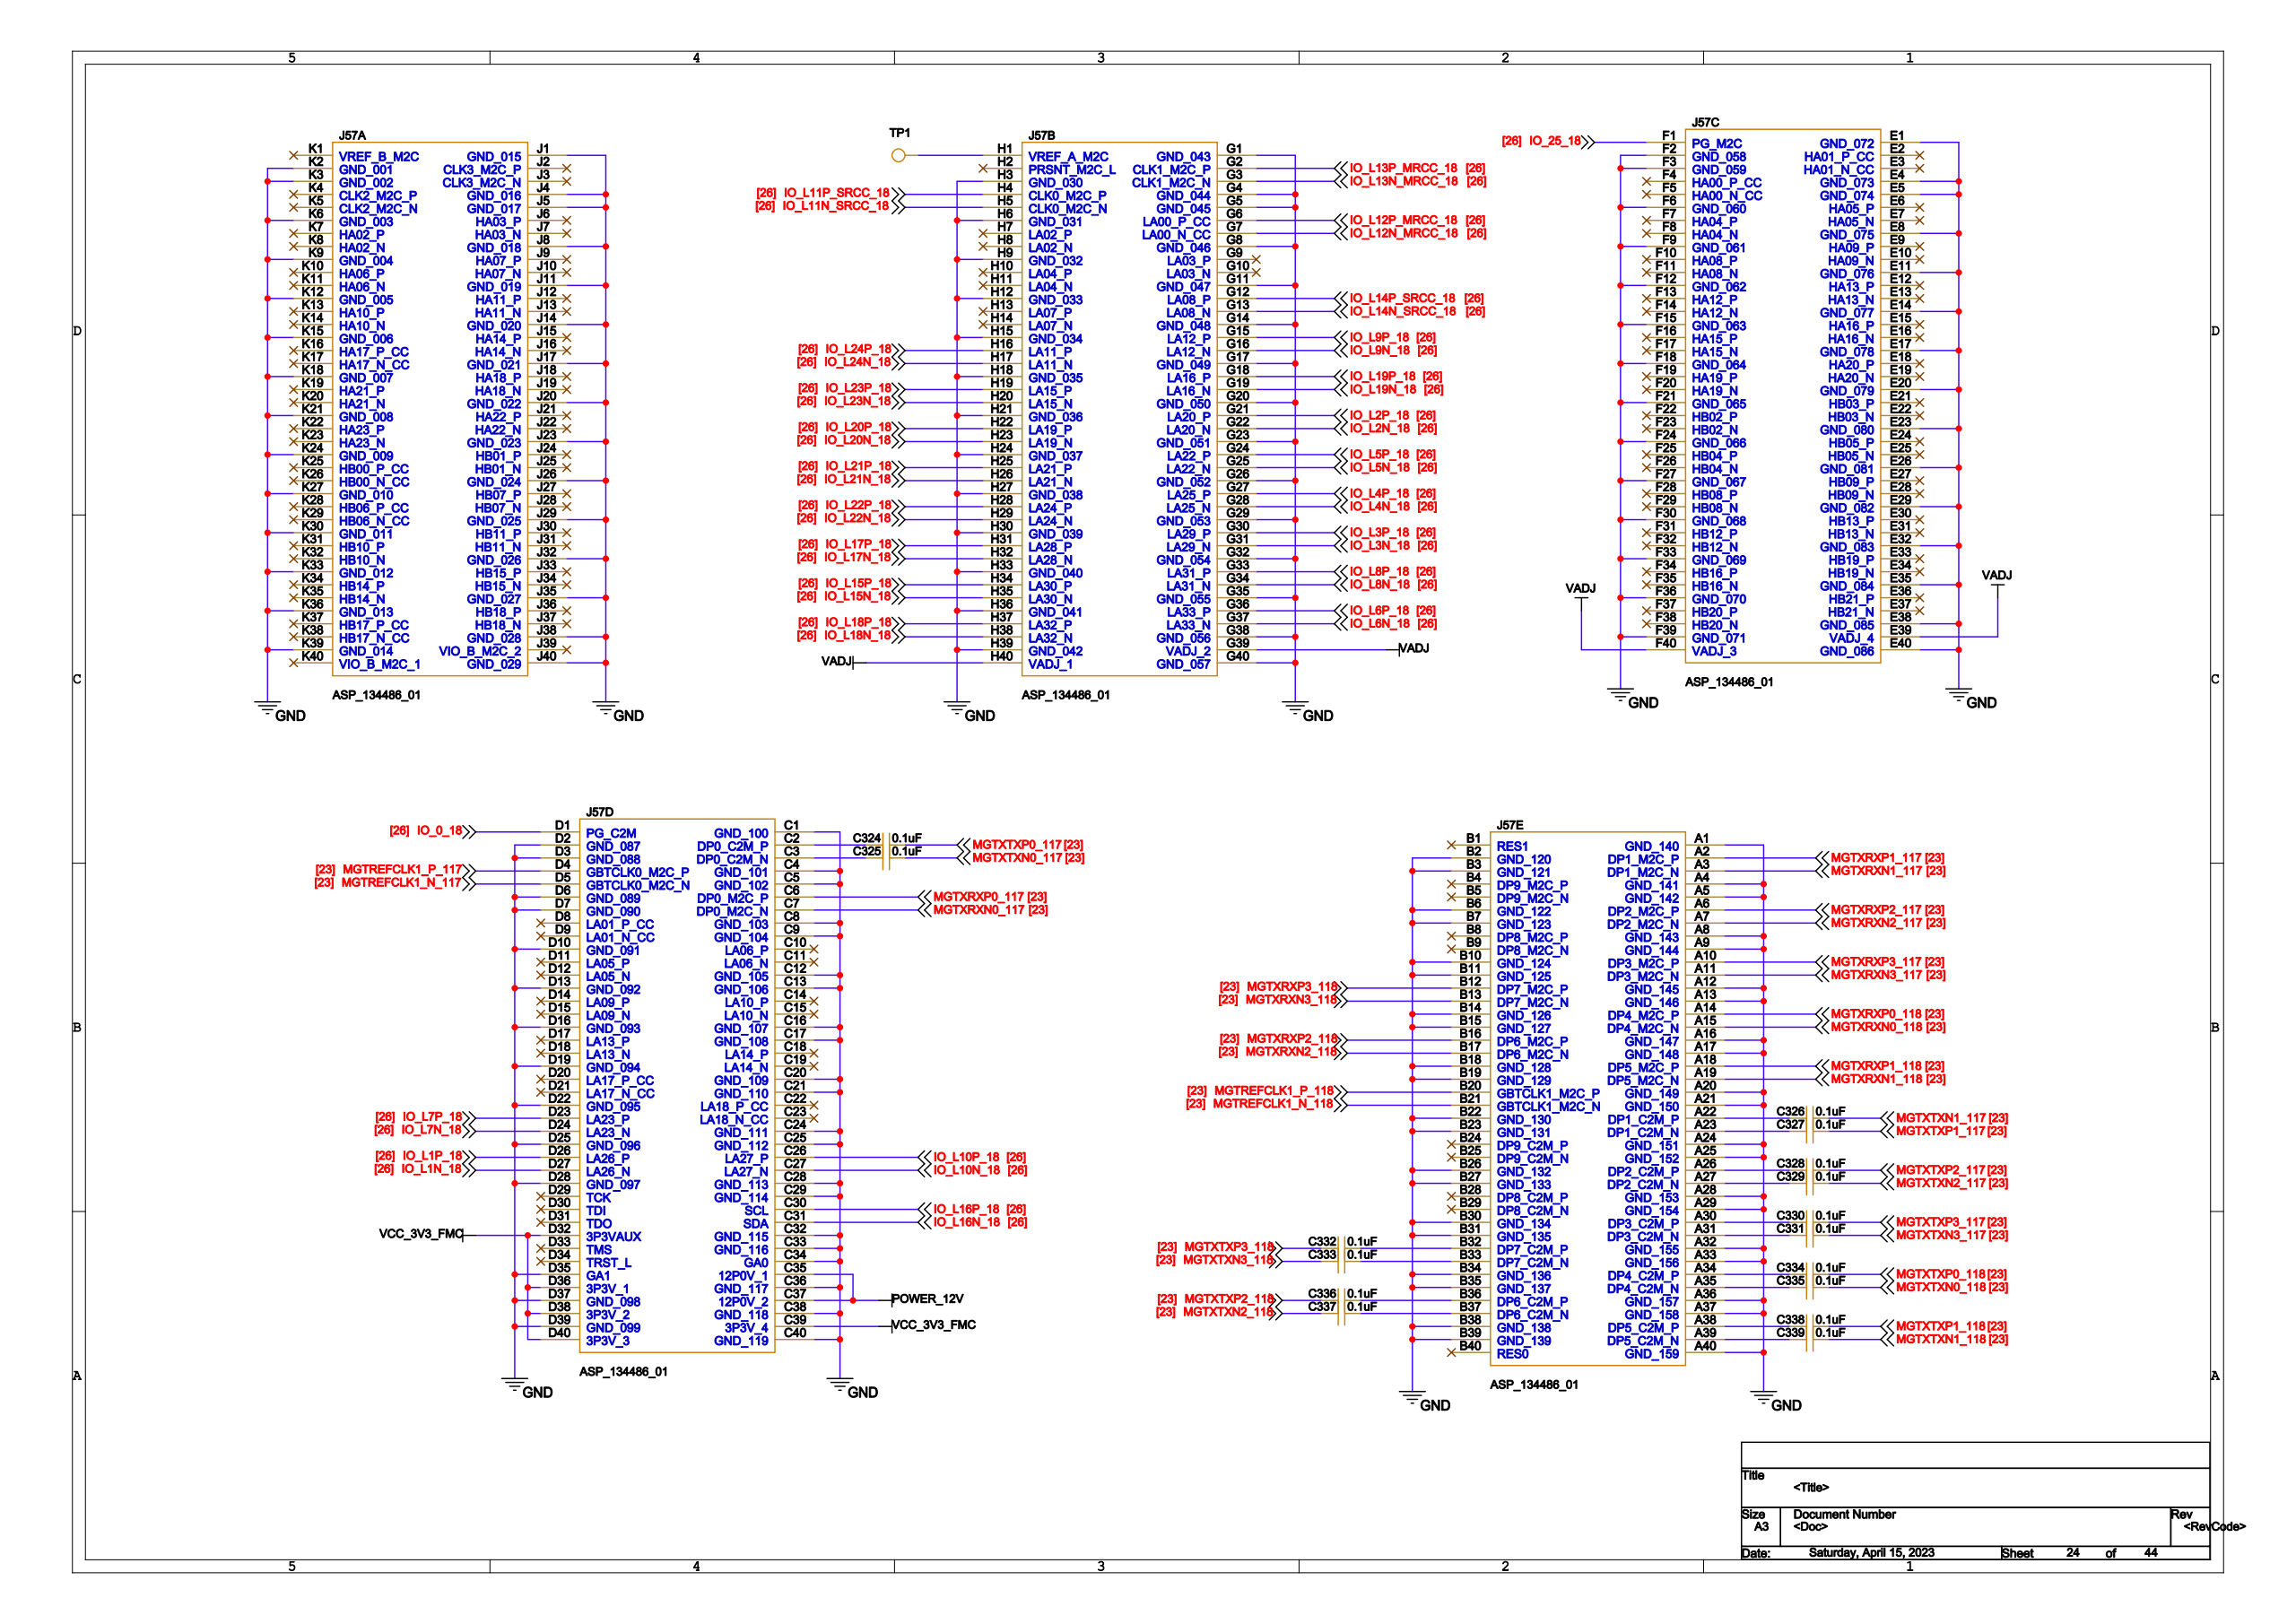Circuit board | Cadence Allegro | 1034 parts | 912 nets | one sheet of the schematic
Parts on this sheet (reference | value | footprint):
C324 | 0.1uF | C0402
C325 | 0.1uF | C0402
C326 | 0.1uF | C0402
C327 | 0.1uF | C0402
C328 | 0.1uF | C0402
C329 | 0.1uF | C0402
C330 | 0.1uF | C0402
C331 | 0.1uF | C0402
C332 | 0.1uF | C0402
C333 | 0.1uF | C0402
C334 | 0.1uF | C0402
C335 | 0.1uF | C0402
C336 | 0.1uF | C0402
C337 | 0.1uF | C0402
C338 | 0.1uF | C0402
C339 | 0.1uF | C0402
J57 | ASP_134486_01 | ASP_134486_01
TP1 | T POINT R | SMD_M3
Nets of these parts (net: part-pin ...):
GND: J57-A1 J57-A4 J57-A5 J57-A8 J57-A9 J57-A12 J57-A13 J57-A16 J57-A17 J57-A20 J57-A21 J57-A24 J57-A25 J57-A28 J57-A29 J57-A32 J57-A33 J57-A36 J57-A37 J57-A40 J57-B2 J57-B3 J57-B6 J57-B7 J57-B10 J57-B11 J57-B14 J57-B15 J57-B18 J57-B19 J57-B22 J57-B23 J57-B26 J57-B27 J57-B30 J57-B31 J57-B34 J57-B35 J57-B38 J57-B39 J57-C1 J57-C4 J57-C5 J57-C8 J57-C9 J57-C12 J57-C13 J57-C16 J57-C17 J57-C20 J57-C21 J57-C24 J57-C25 J57-C28 J57-C29 J57-C32 J57-C33 J57-C34 J57-C36 J57-C38 J57-C40 J57-D2 J57-D3 J57-D6 J57-D7 J57-D10 J57-D13 J57-D16 J57-D19 J57-D22 J57-D25 J57-D28 J57-D35 J57-D37 J57-D39 J57-E1 J57-E4 J57-E5 J57-E8 J57-E11 J57-E14 J57-E17 J57-E20 J57-E23 J57-E26 J57-E29 J57-E32 J57-E35 J57-E38 J57-E40 J57-F2 J57-F3 J57-F6 J57-F9 J57-F12 J57-F15 J57-F18 J57-F21 J57-F24 J57-F27 J57-F30 J57-F33 J57-F36 J57-F39 J57-G1 J57-G4 J57-G5 J57-G8 J57-G11 J57-G14 J57-G17 J57-G20 J57-G23 J57-G26 J57-G29 J57-G32 J57-G35 J57-G38 J57-G40 J57-H3 J57-H6 J57-H9 J57-H12 J57-H15 J57-H18 J57-H21 J57-H24 J57-H27 J57-H30 J57-H33 J57-H36 J57-H39 J57-J1 J57-J4 J57-J5 J57-J8 J57-J11 J57-J14 J57-J17 J57-J20 J57-J23 J57-J26 J57-J29 J57-J32 J57-J35 J57-J38 J57-J40 J57-K2 J57-K3 J57-K6 J57-K9 J57-K12 J57-K15 J57-K18 J57-K21 J57-K24 J57-K27 J57-K30 J57-K33 J57-K36 J57-K39
MGTXTXP1_118: C338-1
N13969847: C338-2 J57-A38
MGTXTXN1_118: C339-1
N13969851: C339-2 J57-A39
MGTXTXN3_117: C331-1
N13861804: C331-2 J57-A31
N13969907: C332-1 J57-B32
MGTXTXP3_118: C332-2
N13969911: C333-1 J57-B33
MGTXTXN3_118: C333-2
MGTXTXP0_118: C334-1
N13969839: C334-2 J57-A34
MGTXTXN0_118: C335-1
N13969843: C335-2 J57-A35
N13969915: C336-1 J57-B36
MGTXTXP2_118: C336-2
N13969919: C337-1 J57-B37
MGTXTXN2_118: C337-2
MGTXRXP3_118: J57-B12
MGTXRXN3_118: J57-B13
MGTXRXP2_118: J57-B16
MGTXRXP3_117: J57-A10
MGTXRXN3_117: J57-A11
MGTXRXP2_117: J57-A6
MGTXRXN2_118: J57-B17
MGTXRXN2_117: J57-A7
MGTREFCLK1_P_118: J57-B20
MGTREFCLK1_P_117: J57-D4
MGTREFCLK1_N_118: J57-B21
MGTREFCLK1_N_117: J57-D5
MGTXRXP1_118: J57-A18
MGTXRXP1_117: J57-A2
MGTXRXN1_118: J57-A19
MGTXRXN1_117: J57-A3
MGTXRXP0_118: J57-A14
MGTXRXP0_117: J57-C6
MGTXRXN0_118: J57-A15
MGTXRXN0_117: J57-C7
MGTXTXP0_117: C324-1
N13861662: C324-2 J57-C2
MGTXTXN0_117: C325-1
N13861664: C325-2 J57-C3
MGTXTXN1_117: C326-1
N13861700: C326-2 J57-A22
MGTXTXP1_117: C327-1
N13861702: C327-2 J57-A23
MGTXTXP2_117: C328-1
N13861758: C328-2 J57-A26
MGTXTXN2_117: C329-1
N13861760: C329-2 J57-A27
MGTXTXP3_117: C330-1
N13861802: C330-2 J57-A30
POWER_12V: J57-C35 J57-C37
IO_L11N_SRCC_18: J57-H5
IO_L11P_SRCC_18: J57-H4
IO_L13N_MRCC_18: J57-G3
IO_L13P_MRCC_18: J57-G2
IO_L12N_MRCC_18: J57-G7
IO_L12P_MRCC_18: J57-G6
IO_L14N_SRCC_18: J57-G13
IO_L14P_SRCC_18: J57-G12
IO_L24N_18: J57-H17
IO_L24P_18: J57-H16
IO_L9N_18: J57-G16
IO_L9P_18: J57-G15
IO_L23N_18: J57-H20
IO_L23P_18: J57-H19
IO_L19N_18: J57-G19
IO_L19P_18: J57-G18
IO_L20N_18: J57-H23
IO_L20P_18: J57-H22
IO_L2N_18: J57-G22
IO_L2P_18: J57-G21
IO_L21N_18: J57-H26
IO_L21P_18: J57-H25
IO_L5N_18: J57-G25
IO_L5P_18: J57-G24
IO_L22N_18: J57-H29
IO_L22P_18: J57-H28
IO_L4N_18: J57-G28
IO_L4P_18: J57-G27
IO_L17N_18: J57-H32
IO_L17P_18: J57-H31
IO_L3N_18: J57-G31
IO_L3P_18: J57-G30
IO_L15N_18: J57-H35
IO_L15P_18: J57-H34
IO_L8N_18: J57-G34
IO_L8P_18: J57-G33
IO_L18N_18: J57-H38
IO_L18P_18: J57-H37
IO_L6N_18: J57-G37
IO_L6P_18: J57-G36
VADJ: J57-E39 J57-F40 J57-G39 J57-H40
N13997613: TP1-1 J57-H1
IO_25_18: J57-F1
VCC_3V3_FMC: J57-C39 J57-D32 J57-D36 J57-D38 J57-D40
IO_L7N_18: J57-D24
IO_L7P_18: J57-D23
IO_L1N_18: J57-D27
IO_L1P_18: J57-D26
IO_L10N_18: J57-C27
IO_L10P_18: J57-C26
IO_0_18: J57-D1
IO_L16P_18: J57-C30
IO_L16N_18: J57-C31